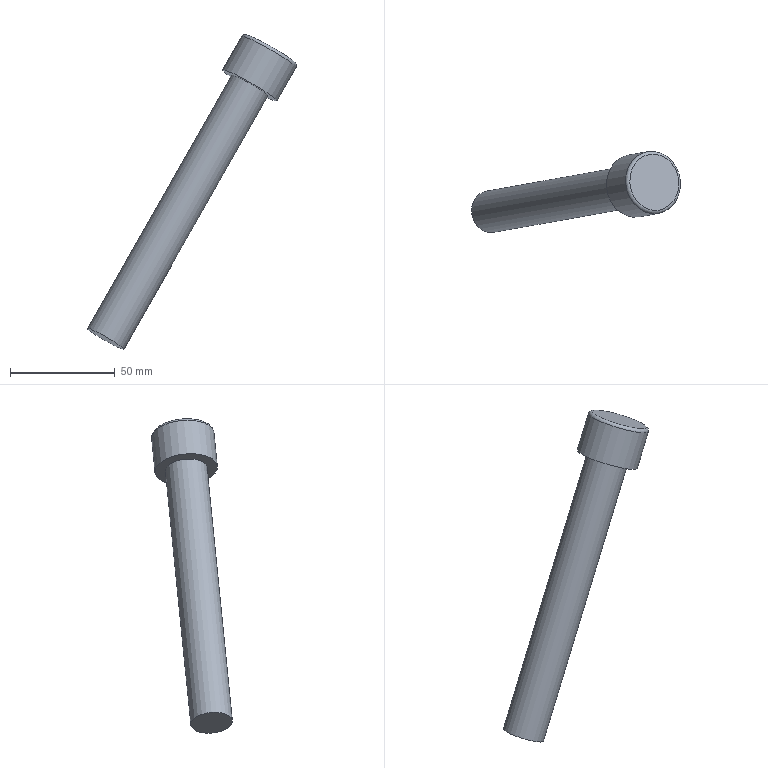Part | NX | features solid 2 | 1 solid | 6 faces | box 100 x 38.673 x 150.515 mm | volume 58075 mm3 | plane 3 | cylinder 2 | torus 1 | commonest cylinder face diameters 20 x1 30 x1
STEP:
#1=CARTESIAN_POINT('',(1034.436,-51.895,-37.081));
#2=VERTEX_POINT('',#1);
#3=CARTESIAN_POINT('',(1025.743,-51.895,-32.138));
#4=DIRECTION('',(0.4924,0.08682,0.866));
#5=DIRECTION('',(0.8693,0.,-0.4943));
#6=AXIS2_PLACEMENT_3D('',#3,#4,#5);
#7=CIRCLE('',#6,10.);
#8=EDGE_CURVE('',#2,#2,#7,.F.);
#9=ORIENTED_EDGE('',*,*,#8,.T.);
#10=EDGE_LOOP('',(#9));
#11=FACE_BOUND('',#10,.T.);
#12=CARTESIAN_POINT('',(1025.743,-51.895,-32.138));
#13=DIRECTION('',(0.4924,0.08682,0.866));
#14=DIRECTION('',(0.1736,-0.9848,0.));
#15=AXIS2_PLACEMENT_3D('',#12,#13,#14);
#16=PLANE('',#15);
#17=ADVANCED_FACE('',(#11),#16,.F.);
#18=ORIENTED_EDGE('',*,*,#8,.F.);
#19=EDGE_LOOP('',(#18));
#20=FACE_BOUND('',#19,.T.);
#21=CARTESIAN_POINT('',(1096.416,-49.587,89.106));
#22=VERTEX_POINT('',#21);
#23=CARTESIAN_POINT('',(1094.68,-39.739,89.106));
#24=DIRECTION('',(-0.4924,-0.08682,-0.866));
#25=DIRECTION('',(0.1736,-0.9848,0.));
#26=AXIS2_PLACEMENT_3D('',#23,#24,#25);
#27=CIRCLE('',#26,10.);
#28=EDGE_CURVE('',#22,#22,#27,.T.);
#29=ORIENTED_EDGE('',*,*,#28,.T.);
#30=EDGE_LOOP('',(#29));
#31=FACE_BOUND('',#30,.T.);
#32=CARTESIAN_POINT('',(1124.224,-34.53,141.067));
#33=DIRECTION('',(-0.4924,-0.08682,-0.866));
#34=DIRECTION('',(-0.1736,0.9848,0.));
#35=AXIS2_PLACEMENT_3D('',#32,#33,#34);
#36=CYLINDRICAL_SURFACE('',#35,10.);
#37=ADVANCED_FACE('',(#20,#31),#36,.T.);
#38=CARTESIAN_POINT('',(1097.285,-54.511,89.106));
#39=VERTEX_POINT('',#38);
#40=CARTESIAN_POINT('',(1094.68,-39.739,89.106));
#41=DIRECTION('',(-0.4924,-0.08682,-0.866));
#42=DIRECTION('',(0.1736,-0.9848,0.));
#43=AXIS2_PLACEMENT_3D('',#40,#41,#42);
#44=CIRCLE('',#43,15.);
#45=EDGE_CURVE('',#39,#39,#44,.T.);
#46=ORIENTED_EDGE('',*,*,#45,.T.);
#47=EDGE_LOOP('',(#46));
#48=FACE_BOUND('',#47,.T.);
#49=ORIENTED_EDGE('',*,*,#28,.F.);
#50=EDGE_LOOP('',(#49));
#51=FACE_BOUND('',#50,.T.);
#52=CARTESIAN_POINT('',(1094.68,-39.739,89.106));
#53=DIRECTION('',(0.4924,0.08682,0.866));
#54=DIRECTION('',(0.1736,-0.9848,0.));
#55=AXIS2_PLACEMENT_3D('',#52,#53,#54);
#56=PLANE('',#55);
#57=ADVANCED_FACE('',(#48,#51),#56,.F.);
#58=CARTESIAN_POINT('',(1106.394,-52.905,105.127));
#59=VERTEX_POINT('',#58);
#60=CARTESIAN_POINT('',(1103.789,-38.133,105.127));
#61=DIRECTION('',(-0.4924,-0.08682,-0.866));
#62=DIRECTION('',(0.1736,-0.9848,0.));
#63=AXIS2_PLACEMENT_3D('',#60,#61,#62);
#64=CIRCLE('',#63,15.);
#65=EDGE_CURVE('',#59,#59,#64,.F.);
#66=ORIENTED_EDGE('',*,*,#65,.F.);
#67=EDGE_LOOP('',(#66));
#68=FACE_BOUND('',#67,.T.);
#69=ORIENTED_EDGE('',*,*,#45,.F.);
#70=EDGE_LOOP('',(#69));
#71=FACE_BOUND('',#70,.T.);
#72=CARTESIAN_POINT('',(1094.68,-39.739,89.106));
#73=DIRECTION('',(0.4924,0.08682,0.866));
#74=DIRECTION('',(0.1736,-0.9848,0.));
#75=AXIS2_PLACEMENT_3D('',#72,#73,#74);
#76=CYLINDRICAL_SURFACE('',#75,15.);
#77=ADVANCED_FACE('',(#68,#71),#76,.T.);
#78=CARTESIAN_POINT('',(1106.872,-51.298,106.426));
#79=VERTEX_POINT('',#78);
#80=CARTESIAN_POINT('',(1104.528,-38.003,106.426));
#81=DIRECTION('',(-0.4924,-0.08682,-0.866));
#82=DIRECTION('',(0.1736,-0.9848,0.));
#83=AXIS2_PLACEMENT_3D('',#80,#81,#82);
#84=CIRCLE('',#83,13.5);
#85=EDGE_CURVE('',#79,#79,#84,.T.);
#86=ORIENTED_EDGE('',*,*,#85,.F.);
#87=EDGE_LOOP('',(#86));
#88=FACE_BOUND('',#87,.T.);
#89=CARTESIAN_POINT('',(1104.528,-38.003,106.426));
#90=DIRECTION('',(0.4924,0.08682,0.866));
#91=DIRECTION('',(0.1736,-0.9848,0.));
#92=AXIS2_PLACEMENT_3D('',#89,#90,#91);
#93=PLANE('',#92);
#94=ADVANCED_FACE('',(#88),#93,.T.);
#95=ORIENTED_EDGE('',*,*,#65,.T.);
#96=EDGE_LOOP('',(#95));
#97=FACE_BOUND('',#96,.T.);
#98=ORIENTED_EDGE('',*,*,#85,.T.);
#99=EDGE_LOOP('',(#98));
#100=FACE_BOUND('',#99,.T.);
#101=CARTESIAN_POINT('',(1103.789,-38.133,105.127));
#102=DIRECTION('',(0.4924,0.08682,0.866));
#103=DIRECTION('',(0.1736,-0.9848,0.));
#104=AXIS2_PLACEMENT_3D('',#101,#102,#103);
#105=TOROIDAL_SURFACE('',#104,13.5,1.5);
#106=ADVANCED_FACE('',(#97,#100),#105,.T.);
#107=CLOSED_SHELL('',(#17,#37,#57,#77,#94,#106));
#108=MANIFOLD_SOLID_BREP('',#107);
#109=(LENGTH_UNIT()NAMED_UNIT(*)SI_UNIT(.MILLI.,.METRE.));
#110=UNCERTAINTY_MEASURE_WITH_UNIT(LENGTH_MEASURE(0.00001),#109,'','');
#111=(NAMED_UNIT(*)PLANE_ANGLE_UNIT()SI_UNIT($,.RADIAN.));
#112=(NAMED_UNIT(*)SI_UNIT($,.STERADIAN.)SOLID_ANGLE_UNIT());
#113=(GEOMETRIC_REPRESENTATION_CONTEXT(3)GLOBAL_UNCERTAINTY_ASSIGNED_CONTEXT((#110))GLOBAL_UNIT_ASSIGNED_CONTEXT((#109,#111,#112))REPRESENTATION_CONTEXT('',''));
#114=ADVANCED_BREP_SHAPE_REPRESENTATION('',(#108),#113);